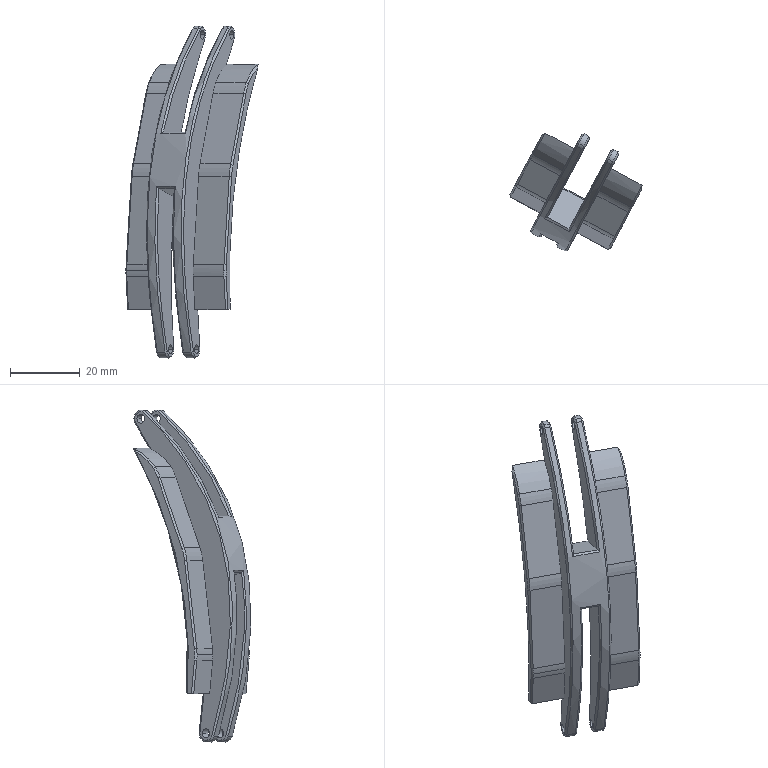Part | SolidWorks | features Chamfer 5, HoleWzd 4, RefSurface 2, ThickenCut 2, BaseBody 1, Fillet 1 | 1 solid | 93 faces | box 37.754 x 33.673 x 94.864 mm | volume 10570 mm3 | plane 28 | cylinder 23 | cone 21 | spline 21 | commonest cylinder face diameters 30 x9 2.5 x8 5 x6